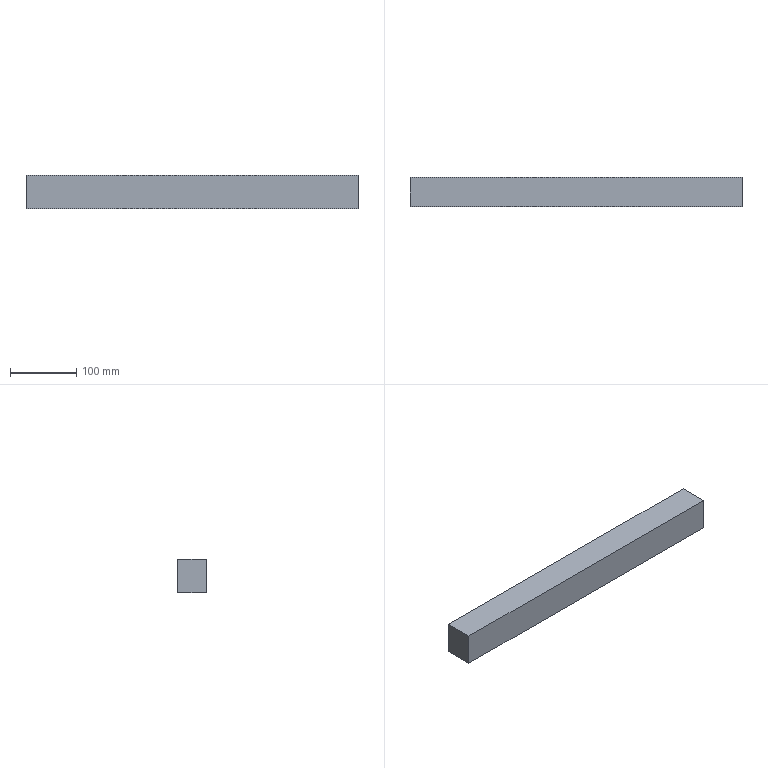Part | SolidWorks | features BaseBody 1 | 1 solid | 6 faces | box 500 x 43.66 x 50 mm | volume 1091500 mm3 | plane 6
STEP:
#1=CARTESIAN_POINT('',(0.,-38.039,25.753));
#2=VERTEX_POINT('',#1);
#3=CARTESIAN_POINT('',(0.,-38.039,-24.247));
#4=VERTEX_POINT('',#3);
#5=CARTESIAN_POINT('',(0.,-38.039,25.753));
#6=DIRECTION('',(0.,0.,-1.));
#7=VECTOR('',#6,1000.);
#8=LINE('',#5,#7);
#9=EDGE_CURVE('',#2,#4,#8,.T.);
#10=ORIENTED_EDGE('',*,*,#9,.T.);
#11=CARTESIAN_POINT('',(500.,-38.039,-24.247));
#12=VERTEX_POINT('',#11);
#13=CARTESIAN_POINT('',(500.,-38.039,-24.247));
#14=DIRECTION('',(-1.,0.,0.));
#15=VECTOR('',#14,1000.);
#16=LINE('',#13,#15);
#17=EDGE_CURVE('',#12,#4,#16,.T.);
#18=ORIENTED_EDGE('',*,*,#17,.F.);
#19=CARTESIAN_POINT('',(500.,-38.039,25.753));
#20=VERTEX_POINT('',#19);
#21=CARTESIAN_POINT('',(500.,-38.039,25.753));
#22=DIRECTION('',(0.,0.,-1.));
#23=VECTOR('',#22,1000.);
#24=LINE('',#21,#23);
#25=EDGE_CURVE('',#20,#12,#24,.T.);
#26=ORIENTED_EDGE('',*,*,#25,.F.);
#27=CARTESIAN_POINT('',(500.,-38.039,25.753));
#28=DIRECTION('',(-1.,0.,0.));
#29=VECTOR('',#28,1000.);
#30=LINE('',#27,#29);
#31=EDGE_CURVE('',#20,#2,#30,.T.);
#32=ORIENTED_EDGE('',*,*,#31,.T.);
#33=EDGE_LOOP('',(#10,#18,#26,#32));
#34=FACE_OUTER_BOUND('',#33,.T.);
#35=CARTESIAN_POINT('',(500.,-38.039,25.753));
#36=DIRECTION('',(0.,1.,0.));
#37=DIRECTION('',(0.,0.,1.));
#38=AXIS2_PLACEMENT_3D('',#35,#36,#37);
#39=PLANE('',#38);
#40=ADVANCED_FACE('',(#34),#39,.F.);
#41=CARTESIAN_POINT('',(0.,5.621,-24.247));
#42=VERTEX_POINT('',#41);
#43=CARTESIAN_POINT('',(0.,-38.039,-24.247));
#44=DIRECTION('',(0.,1.,0.));
#45=VECTOR('',#44,1000.);
#46=LINE('',#43,#45);
#47=EDGE_CURVE('',#4,#42,#46,.T.);
#48=ORIENTED_EDGE('',*,*,#47,.T.);
#49=CARTESIAN_POINT('',(500.,5.621,-24.247));
#50=VERTEX_POINT('',#49);
#51=CARTESIAN_POINT('',(0.,5.621,-24.247));
#52=DIRECTION('',(1.,0.,0.));
#53=VECTOR('',#52,1000.);
#54=LINE('',#51,#53);
#55=EDGE_CURVE('',#42,#50,#54,.T.);
#56=ORIENTED_EDGE('',*,*,#55,.T.);
#57=CARTESIAN_POINT('',(500.,-38.039,-24.247));
#58=DIRECTION('',(0.,1.,0.));
#59=VECTOR('',#58,1000.);
#60=LINE('',#57,#59);
#61=EDGE_CURVE('',#12,#50,#60,.T.);
#62=ORIENTED_EDGE('',*,*,#61,.F.);
#63=ORIENTED_EDGE('',*,*,#17,.T.);
#64=EDGE_LOOP('',(#48,#56,#62,#63));
#65=FACE_OUTER_BOUND('',#64,.T.);
#66=CARTESIAN_POINT('',(500.,-38.039,-24.247));
#67=DIRECTION('',(0.,0.,1.));
#68=DIRECTION('',(1.,0.,0.));
#69=AXIS2_PLACEMENT_3D('',#66,#67,#68);
#70=PLANE('',#69);
#71=ADVANCED_FACE('',(#65),#70,.F.);
#72=CARTESIAN_POINT('',(500.,5.621,25.753));
#73=VERTEX_POINT('',#72);
#74=CARTESIAN_POINT('',(500.,-38.039,25.753));
#75=DIRECTION('',(0.,-1.,0.));
#76=VECTOR('',#75,1000.);
#77=LINE('',#74,#76);
#78=EDGE_CURVE('',#73,#20,#77,.T.);
#79=ORIENTED_EDGE('',*,*,#78,.F.);
#80=CARTESIAN_POINT('',(0.,5.621,25.753));
#81=VERTEX_POINT('',#80);
#82=CARTESIAN_POINT('',(0.,5.621,25.753));
#83=DIRECTION('',(1.,0.,0.));
#84=VECTOR('',#83,1000.);
#85=LINE('',#82,#84);
#86=EDGE_CURVE('',#81,#73,#85,.T.);
#87=ORIENTED_EDGE('',*,*,#86,.F.);
#88=CARTESIAN_POINT('',(0.,-38.039,25.753));
#89=DIRECTION('',(0.,-1.,0.));
#90=VECTOR('',#89,1000.);
#91=LINE('',#88,#90);
#92=EDGE_CURVE('',#81,#2,#91,.T.);
#93=ORIENTED_EDGE('',*,*,#92,.T.);
#94=ORIENTED_EDGE('',*,*,#31,.F.);
#95=EDGE_LOOP('',(#79,#87,#93,#94));
#96=FACE_OUTER_BOUND('',#95,.T.);
#97=CARTESIAN_POINT('',(500.,-38.039,25.753));
#98=DIRECTION('',(0.,0.,-1.));
#99=DIRECTION('',(-1.,0.,0.));
#100=AXIS2_PLACEMENT_3D('',#97,#98,#99);
#101=PLANE('',#100);
#102=ADVANCED_FACE('',(#96),#101,.F.);
#103=CARTESIAN_POINT('',(500.,5.621,25.753));
#104=DIRECTION('',(0.,0.,-1.));
#105=VECTOR('',#104,1000.);
#106=LINE('',#103,#105);
#107=EDGE_CURVE('',#73,#50,#106,.T.);
#108=ORIENTED_EDGE('',*,*,#107,.F.);
#109=ORIENTED_EDGE('',*,*,#78,.T.);
#110=ORIENTED_EDGE('',*,*,#25,.T.);
#111=ORIENTED_EDGE('',*,*,#61,.T.);
#112=EDGE_LOOP('',(#108,#109,#110,#111));
#113=FACE_OUTER_BOUND('',#112,.T.);
#114=CARTESIAN_POINT('',(500.,0.,0.));
#115=DIRECTION('',(1.,0.,0.));
#116=DIRECTION('',(0.,0.,-1.));
#117=AXIS2_PLACEMENT_3D('',#114,#115,#116);
#118=PLANE('',#117);
#119=ADVANCED_FACE('',(#113),#118,.T.);
#120=ORIENTED_EDGE('',*,*,#92,.F.);
#121=CARTESIAN_POINT('',(0.,5.621,25.753));
#122=DIRECTION('',(0.,0.,-1.));
#123=VECTOR('',#122,1000.);
#124=LINE('',#121,#123);
#125=EDGE_CURVE('',#81,#42,#124,.T.);
#126=ORIENTED_EDGE('',*,*,#125,.T.);
#127=ORIENTED_EDGE('',*,*,#47,.F.);
#128=ORIENTED_EDGE('',*,*,#9,.F.);
#129=EDGE_LOOP('',(#120,#126,#127,#128));
#130=FACE_OUTER_BOUND('',#129,.T.);
#131=CARTESIAN_POINT('',(0.,0.,0.));
#132=DIRECTION('',(1.,0.,0.));
#133=DIRECTION('',(0.,0.,-1.));
#134=AXIS2_PLACEMENT_3D('',#131,#132,#133);
#135=PLANE('',#134);
#136=ADVANCED_FACE('',(#130),#135,.F.);
#137=ORIENTED_EDGE('',*,*,#107,.T.);
#138=ORIENTED_EDGE('',*,*,#55,.F.);
#139=ORIENTED_EDGE('',*,*,#125,.F.);
#140=ORIENTED_EDGE('',*,*,#86,.T.);
#141=EDGE_LOOP('',(#137,#138,#139,#140));
#142=FACE_OUTER_BOUND('',#141,.T.);
#143=CARTESIAN_POINT('',(0.,5.621,25.753));
#144=DIRECTION('',(0.,-1.,0.));
#145=DIRECTION('',(0.,0.,-1.));
#146=AXIS2_PLACEMENT_3D('',#143,#144,#145);
#147=PLANE('',#146);
#148=ADVANCED_FACE('',(#142),#147,.F.);
#149=CLOSED_SHELL('',(#40,#71,#102,#119,#136,#148));
#150=MANIFOLD_SOLID_BREP('',#149);
#151=CARTESIAN_POINT('',(0.,0.,0.));
#152=DIRECTION('',(0.,0.,1.));
#153=DIRECTION('',(1.,0.,0.));
#154=AXIS2_PLACEMENT_3D('',#151,#152,#153);
#155=(LENGTH_UNIT()NAMED_UNIT(*)SI_UNIT(.MILLI.,.METRE.));
#156=UNCERTAINTY_MEASURE_WITH_UNIT(LENGTH_MEASURE(0.00001),#155,'','');
#157=(NAMED_UNIT(*)PLANE_ANGLE_UNIT()SI_UNIT($,.RADIAN.));
#158=(NAMED_UNIT(*)SI_UNIT($,.STERADIAN.)SOLID_ANGLE_UNIT());
#159=(GEOMETRIC_REPRESENTATION_CONTEXT(3)GLOBAL_UNCERTAINTY_ASSIGNED_CONTEXT((#156))GLOBAL_UNIT_ASSIGNED_CONTEXT((#155,#157,#158))REPRESENTATION_CONTEXT('',''));
#160=ADVANCED_BREP_SHAPE_REPRESENTATION('',(#150,#154),#159);